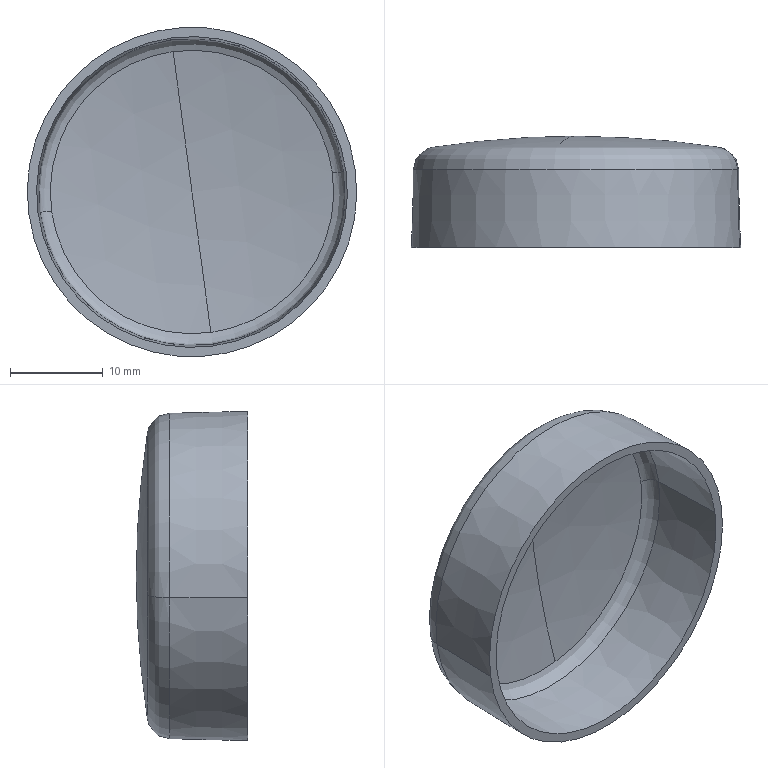Part | SolidWorks | features BaseBody 1 | 1 solid | 13 faces | box 35.5 x 12 x 35.5 mm | volume 1936 mm3 | cone 4 | torus 4 | sphere 4 | plane 1
STEP:
#1=CARTESIAN_POINT('',(53.884,-51.605,2.336));
#2=VERTEX_POINT('',#1);
#3=CARTESIAN_POINT('',(19.116,-51.605,-2.336));
#4=VERTEX_POINT('',#3);
#5=CARTESIAN_POINT('',(36.5,-51.605,0.));
#6=DIRECTION('',(0.,1.,0.));
#7=DIRECTION('',(0.9911,0.,0.1332));
#8=AXIS2_PLACEMENT_3D('',#5,#6,#7);
#9=CIRCLE('',#8,17.54);
#10=EDGE_CURVE('',#2,#4,#9,.T.);
#11=ORIENTED_EDGE('',*,*,#10,.F.);
#12=CARTESIAN_POINT('',(54.092,-60.,2.364));
#13=VERTEX_POINT('',#12);
#14=CARTESIAN_POINT('',(54.092,-60.,2.364));
#15=DIRECTION('',(0.02477,-0.9997,0.003329));
#16=VECTOR('',#15,1000.);
#17=LINE('',#14,#16);
#18=EDGE_CURVE('',#2,#13,#17,.T.);
#19=ORIENTED_EDGE('',*,*,#18,.T.);
#20=CARTESIAN_POINT('',(18.908,-60.,-2.364));
#21=VERTEX_POINT('',#20);
#22=CARTESIAN_POINT('',(36.5,-60.,0.));
#23=DIRECTION('',(0.,1.,0.));
#24=DIRECTION('',(0.9911,0.,0.1332));
#25=AXIS2_PLACEMENT_3D('',#22,#23,#24);
#26=CIRCLE('',#25,17.75);
#27=EDGE_CURVE('',#13,#21,#26,.T.);
#28=ORIENTED_EDGE('',*,*,#27,.T.);
#29=CARTESIAN_POINT('',(18.908,-60.,-2.364));
#30=DIRECTION('',(-0.02477,-0.9997,-0.003329));
#31=VECTOR('',#30,1000.);
#32=LINE('',#29,#31);
#33=EDGE_CURVE('',#4,#21,#32,.T.);
#34=ORIENTED_EDGE('',*,*,#33,.F.);
#35=EDGE_LOOP('',(#11,#19,#28,#34));
#36=FACE_OUTER_BOUND('',#35,.T.);
#37=CARTESIAN_POINT('',(36.5,-60.,0.));
#38=DIRECTION('',(0.,-1.,0.));
#39=DIRECTION('',(-0.9911,0.,-0.1332));
#40=AXIS2_PLACEMENT_3D('',#37,#38,#39);
#41=CONICAL_SURFACE('',#40,17.75,0.02499);
#42=ADVANCED_FACE('',(#36),#41,.T.);
#43=CARTESIAN_POINT('',(20.107,-51.63,-2.203));
#44=VERTEX_POINT('',#43);
#45=CARTESIAN_POINT('',(52.893,-51.63,2.203));
#46=VERTEX_POINT('',#45);
#47=CARTESIAN_POINT('',(36.5,-51.63,0.));
#48=DIRECTION('',(0.,1.,0.));
#49=DIRECTION('',(0.9911,0.,0.1332));
#50=AXIS2_PLACEMENT_3D('',#47,#48,#49);
#51=CIRCLE('',#50,16.54);
#52=EDGE_CURVE('',#44,#46,#51,.T.);
#53=ORIENTED_EDGE('',*,*,#52,.T.);
#54=CARTESIAN_POINT('',(53.1,-60.,2.231));
#55=VERTEX_POINT('',#54);
#56=CARTESIAN_POINT('',(52.893,-51.63,2.203));
#57=DIRECTION('',(0.02477,-0.9997,0.003329));
#58=VECTOR('',#57,1000.);
#59=LINE('',#56,#58);
#60=EDGE_CURVE('',#46,#55,#59,.T.);
#61=ORIENTED_EDGE('',*,*,#60,.T.);
#62=CARTESIAN_POINT('',(19.9,-60.,-2.231));
#63=VERTEX_POINT('',#62);
#64=CARTESIAN_POINT('',(36.5,-60.,0.));
#65=DIRECTION('',(0.,1.,0.));
#66=DIRECTION('',(0.9911,0.,0.1332));
#67=AXIS2_PLACEMENT_3D('',#64,#65,#66);
#68=CIRCLE('',#67,16.75);
#69=EDGE_CURVE('',#63,#55,#68,.T.);
#70=ORIENTED_EDGE('',*,*,#69,.F.);
#71=CARTESIAN_POINT('',(20.107,-51.63,-2.203));
#72=DIRECTION('',(-0.02477,-0.9997,-0.003329));
#73=VECTOR('',#72,1000.);
#74=LINE('',#71,#73);
#75=EDGE_CURVE('',#44,#63,#74,.T.);
#76=ORIENTED_EDGE('',*,*,#75,.F.);
#77=EDGE_LOOP('',(#53,#61,#70,#76));
#78=FACE_OUTER_BOUND('',#77,.T.);
#79=CARTESIAN_POINT('',(36.5,-51.63,0.));
#80=DIRECTION('',(0.,-1.,0.));
#81=DIRECTION('',(-0.9911,0.,-0.1332));
#82=AXIS2_PLACEMENT_3D('',#79,#80,#81);
#83=CONICAL_SURFACE('',#82,16.54,0.02499);
#84=ADVANCED_FACE('',(#78),#83,.F.);
#85=ORIENTED_EDGE('',*,*,#52,.F.);
#86=CARTESIAN_POINT('',(21.364,-50.185,-2.034));
#87=VERTEX_POINT('',#86);
#88=CARTESIAN_POINT('',(21.593,-51.667,-2.003));
#89=DIRECTION('',(0.1332,0.,-0.9911));
#90=DIRECTION('',(-0.9911,0.,-0.1332));
#91=AXIS2_PLACEMENT_3D('',#88,#89,#90);
#92=CIRCLE('',#91,1.5);
#93=EDGE_CURVE('',#44,#87,#92,.T.);
#94=ORIENTED_EDGE('',*,*,#93,.T.);
#95=CARTESIAN_POINT('',(34.466,-50.185,15.136));
#96=VERTEX_POINT('',#95);
#97=CARTESIAN_POINT('',(36.5,-50.185,0.));
#98=DIRECTION('',(0.,1.,0.));
#99=DIRECTION('',(0.9911,0.,0.1332));
#100=AXIS2_PLACEMENT_3D('',#97,#98,#99);
#101=CIRCLE('',#100,15.272);
#102=EDGE_CURVE('',#87,#96,#101,.T.);
#103=ORIENTED_EDGE('',*,*,#102,.T.);
#104=CARTESIAN_POINT('',(51.636,-50.185,2.034));
#105=VERTEX_POINT('',#104);
#106=CARTESIAN_POINT('',(36.5,-50.185,0.));
#107=DIRECTION('',(0.,1.,0.));
#108=DIRECTION('',(0.9911,0.,0.1332));
#109=AXIS2_PLACEMENT_3D('',#106,#107,#108);
#110=CIRCLE('',#109,15.272);
#111=EDGE_CURVE('',#96,#105,#110,.T.);
#112=ORIENTED_EDGE('',*,*,#111,.T.);
#113=CARTESIAN_POINT('',(51.407,-51.667,2.003));
#114=DIRECTION('',(-0.1332,0.,0.9911));
#115=DIRECTION('',(0.9911,0.,0.1332));
#116=AXIS2_PLACEMENT_3D('',#113,#114,#115);
#117=CIRCLE('',#116,1.5);
#118=EDGE_CURVE('',#46,#105,#117,.T.);
#119=ORIENTED_EDGE('',*,*,#118,.F.);
#120=EDGE_LOOP('',(#85,#94,#103,#112,#119));
#121=FACE_OUTER_BOUND('',#120,.T.);
#122=CARTESIAN_POINT('',(36.5,-51.667,0.));
#123=DIRECTION('',(0.,1.,0.));
#124=DIRECTION('',(0.9911,0.,0.1332));
#125=AXIS2_PLACEMENT_3D('',#122,#123,#124);
#126=TOROIDAL_SURFACE('',#125,15.041,1.5);
#127=ADVANCED_FACE('',(#121),#126,.F.);
#128=CARTESIAN_POINT('',(38.534,-50.185,-15.136));
#129=VERTEX_POINT('',#128);
#130=CARTESIAN_POINT('',(36.5,-50.185,0.));
#131=DIRECTION('',(0.,1.,0.));
#132=DIRECTION('',(0.9911,0.,0.1332));
#133=AXIS2_PLACEMENT_3D('',#130,#131,#132);
#134=CIRCLE('',#133,15.272);
#135=EDGE_CURVE('',#129,#87,#134,.T.);
#136=ORIENTED_EDGE('',*,*,#135,.F.);
#137=CARTESIAN_POINT('',(36.5,-49.,0.));
#138=VERTEX_POINT('',#137);
#139=CARTESIAN_POINT('',(36.5,-148.,0.));
#140=DIRECTION('',(0.9911,0.,0.1332));
#141=DIRECTION('',(0.1332,0.,-0.9911));
#142=AXIS2_PLACEMENT_3D('',#139,#140,#141);
#143=CIRCLE('',#142,99.);
#144=EDGE_CURVE('',#129,#138,#143,.T.);
#145=ORIENTED_EDGE('',*,*,#144,.T.);
#146=CARTESIAN_POINT('',(36.5,-148.,0.));
#147=DIRECTION('',(-0.9911,0.,-0.1332));
#148=DIRECTION('',(-0.1332,0.,0.9911));
#149=AXIS2_PLACEMENT_3D('',#146,#147,#148);
#150=CIRCLE('',#149,99.);
#151=EDGE_CURVE('',#96,#138,#150,.T.);
#152=ORIENTED_EDGE('',*,*,#151,.F.);
#153=ORIENTED_EDGE('',*,*,#102,.F.);
#154=EDGE_LOOP('',(#136,#145,#152,#153));
#155=FACE_OUTER_BOUND('',#154,.T.);
#156=CARTESIAN_POINT('',(36.5,-148.,0.));
#157=DIRECTION('',(0.9911,0.,0.1332));
#158=DIRECTION('',(-0.1332,0.,0.9911));
#159=AXIS2_PLACEMENT_3D('',#156,#157,#158);
#160=SPHERICAL_SURFACE('',#159,99.);
#161=ADVANCED_FACE('',(#155),#160,.F.);
#162=CARTESIAN_POINT('',(21.211,-49.197,-2.055));
#163=VERTEX_POINT('',#162);
#164=CARTESIAN_POINT('',(34.445,-49.197,15.289));
#165=VERTEX_POINT('',#164);
#166=CARTESIAN_POINT('',(36.5,-49.197,0.));
#167=DIRECTION('',(0.,1.,0.));
#168=DIRECTION('',(0.9911,0.,0.1332));
#169=AXIS2_PLACEMENT_3D('',#166,#167,#168);
#170=CIRCLE('',#169,15.427);
#171=EDGE_CURVE('',#163,#165,#170,.T.);
#172=ORIENTED_EDGE('',*,*,#171,.T.);
#173=CARTESIAN_POINT('',(36.5,-48.,0.));
#174=VERTEX_POINT('',#173);
#175=CARTESIAN_POINT('',(36.5,-148.,0.));
#176=DIRECTION('',(-0.9911,0.,-0.1332));
#177=DIRECTION('',(-0.1332,0.,0.9911));
#178=AXIS2_PLACEMENT_3D('',#175,#176,#177);
#179=CIRCLE('',#178,100.);
#180=EDGE_CURVE('',#165,#174,#179,.T.);
#181=ORIENTED_EDGE('',*,*,#180,.T.);
#182=CARTESIAN_POINT('',(38.555,-49.197,-15.289));
#183=VERTEX_POINT('',#182);
#184=CARTESIAN_POINT('',(36.5,-148.,0.));
#185=DIRECTION('',(0.9911,0.,0.1332));
#186=DIRECTION('',(0.1332,0.,-0.9911));
#187=AXIS2_PLACEMENT_3D('',#184,#185,#186);
#188=CIRCLE('',#187,100.);
#189=EDGE_CURVE('',#183,#174,#188,.T.);
#190=ORIENTED_EDGE('',*,*,#189,.F.);
#191=CARTESIAN_POINT('',(36.5,-49.197,0.));
#192=DIRECTION('',(0.,1.,0.));
#193=DIRECTION('',(0.9911,0.,0.1332));
#194=AXIS2_PLACEMENT_3D('',#191,#192,#193);
#195=CIRCLE('',#194,15.427);
#196=EDGE_CURVE('',#183,#163,#195,.T.);
#197=ORIENTED_EDGE('',*,*,#196,.T.);
#198=EDGE_LOOP('',(#172,#181,#190,#197));
#199=FACE_OUTER_BOUND('',#198,.T.);
#200=CARTESIAN_POINT('',(36.5,-148.,0.));
#201=DIRECTION('',(-0.9911,0.,-0.1332));
#202=DIRECTION('',(0.1332,0.,-0.9911));
#203=AXIS2_PLACEMENT_3D('',#200,#201,#202);
#204=SPHERICAL_SURFACE('',#203,100.);
#205=ADVANCED_FACE('',(#199),#204,.T.);
#206=ORIENTED_EDGE('',*,*,#10,.T.);
#207=CARTESIAN_POINT('',(21.593,-51.667,-2.003));
#208=DIRECTION('',(0.1332,0.,-0.9911));
#209=DIRECTION('',(-0.9911,0.,-0.1332));
#210=AXIS2_PLACEMENT_3D('',#207,#208,#209);
#211=CIRCLE('',#210,2.5);
#212=EDGE_CURVE('',#4,#163,#211,.T.);
#213=ORIENTED_EDGE('',*,*,#212,.T.);
#214=ORIENTED_EDGE('',*,*,#196,.F.);
#215=CARTESIAN_POINT('',(51.789,-49.197,2.055));
#216=VERTEX_POINT('',#215);
#217=CARTESIAN_POINT('',(36.5,-49.197,0.));
#218=DIRECTION('',(0.,1.,0.));
#219=DIRECTION('',(0.9911,0.,0.1332));
#220=AXIS2_PLACEMENT_3D('',#217,#218,#219);
#221=CIRCLE('',#220,15.427);
#222=EDGE_CURVE('',#216,#183,#221,.T.);
#223=ORIENTED_EDGE('',*,*,#222,.F.);
#224=CARTESIAN_POINT('',(51.407,-51.667,2.003));
#225=DIRECTION('',(-0.1332,0.,0.9911));
#226=DIRECTION('',(0.9911,0.,0.1332));
#227=AXIS2_PLACEMENT_3D('',#224,#225,#226);
#228=CIRCLE('',#227,2.5);
#229=EDGE_CURVE('',#2,#216,#228,.T.);
#230=ORIENTED_EDGE('',*,*,#229,.F.);
#231=EDGE_LOOP('',(#206,#213,#214,#223,#230));
#232=FACE_OUTER_BOUND('',#231,.T.);
#233=CARTESIAN_POINT('',(36.5,-51.667,0.));
#234=DIRECTION('',(0.,1.,0.));
#235=DIRECTION('',(0.9911,0.,0.1332));
#236=AXIS2_PLACEMENT_3D('',#233,#234,#235);
#237=TOROIDAL_SURFACE('',#236,15.041,2.5);
#238=ADVANCED_FACE('',(#232),#237,.T.);
#239=ORIENTED_EDGE('',*,*,#212,.F.);
#240=CARTESIAN_POINT('',(36.5,-51.605,0.));
#241=DIRECTION('',(0.,1.,0.));
#242=DIRECTION('',(0.9911,0.,0.1332));
#243=AXIS2_PLACEMENT_3D('',#240,#241,#242);
#244=CIRCLE('',#243,17.54);
#245=EDGE_CURVE('',#4,#2,#244,.T.);
#246=ORIENTED_EDGE('',*,*,#245,.T.);
#247=ORIENTED_EDGE('',*,*,#229,.T.);
#248=CARTESIAN_POINT('',(36.5,-49.197,0.));
#249=DIRECTION('',(0.,1.,0.));
#250=DIRECTION('',(0.9911,0.,0.1332));
#251=AXIS2_PLACEMENT_3D('',#248,#249,#250);
#252=CIRCLE('',#251,15.427);
#253=EDGE_CURVE('',#165,#216,#252,.T.);
#254=ORIENTED_EDGE('',*,*,#253,.F.);
#255=ORIENTED_EDGE('',*,*,#171,.F.);
#256=EDGE_LOOP('',(#239,#246,#247,#254,#255));
#257=FACE_OUTER_BOUND('',#256,.T.);
#258=CARTESIAN_POINT('',(36.5,-51.667,0.));
#259=DIRECTION('',(0.,1.,0.));
#260=DIRECTION('',(0.9911,0.,0.1332));
#261=AXIS2_PLACEMENT_3D('',#258,#259,#260);
#262=TOROIDAL_SURFACE('',#261,15.041,2.5);
#263=ADVANCED_FACE('',(#257),#262,.T.);
#264=ORIENTED_EDGE('',*,*,#180,.F.);
#265=ORIENTED_EDGE('',*,*,#253,.T.);
#266=ORIENTED_EDGE('',*,*,#222,.T.);
#267=ORIENTED_EDGE('',*,*,#189,.T.);
#268=EDGE_LOOP('',(#264,#265,#266,#267));
#269=FACE_OUTER_BOUND('',#268,.T.);
#270=CARTESIAN_POINT('',(36.5,-148.,0.));
#271=DIRECTION('',(-0.9911,0.,-0.1332));
#272=DIRECTION('',(0.1332,0.,-0.9911));
#273=AXIS2_PLACEMENT_3D('',#270,#271,#272);
#274=SPHERICAL_SURFACE('',#273,100.);
#275=ADVANCED_FACE('',(#269),#274,.T.);
#276=ORIENTED_EDGE('',*,*,#144,.F.);
#277=CARTESIAN_POINT('',(36.5,-50.185,0.));
#278=DIRECTION('',(0.,1.,0.));
#279=DIRECTION('',(0.9911,0.,0.1332));
#280=AXIS2_PLACEMENT_3D('',#277,#278,#279);
#281=CIRCLE('',#280,15.272);
#282=EDGE_CURVE('',#105,#129,#281,.T.);
#283=ORIENTED_EDGE('',*,*,#282,.F.);
#284=ORIENTED_EDGE('',*,*,#111,.F.);
#285=ORIENTED_EDGE('',*,*,#151,.T.);
#286=EDGE_LOOP('',(#276,#283,#284,#285));
#287=FACE_OUTER_BOUND('',#286,.T.);
#288=CARTESIAN_POINT('',(36.5,-148.,0.));
#289=DIRECTION('',(0.9911,0.,0.1332));
#290=DIRECTION('',(-0.1332,0.,0.9911));
#291=AXIS2_PLACEMENT_3D('',#288,#289,#290);
#292=SPHERICAL_SURFACE('',#291,99.);
#293=ADVANCED_FACE('',(#287),#292,.F.);
#294=ORIENTED_EDGE('',*,*,#93,.F.);
#295=CARTESIAN_POINT('',(36.5,-51.63,0.));
#296=DIRECTION('',(0.,1.,0.));
#297=DIRECTION('',(0.9911,0.,0.1332));
#298=AXIS2_PLACEMENT_3D('',#295,#296,#297);
#299=CIRCLE('',#298,16.54);
#300=EDGE_CURVE('',#46,#44,#299,.T.);
#301=ORIENTED_EDGE('',*,*,#300,.F.);
#302=ORIENTED_EDGE('',*,*,#118,.T.);
#303=ORIENTED_EDGE('',*,*,#282,.T.);
#304=ORIENTED_EDGE('',*,*,#135,.T.);
#305=EDGE_LOOP('',(#294,#301,#302,#303,#304));
#306=FACE_OUTER_BOUND('',#305,.T.);
#307=CARTESIAN_POINT('',(36.5,-51.667,0.));
#308=DIRECTION('',(0.,1.,0.));
#309=DIRECTION('',(0.9911,0.,0.1332));
#310=AXIS2_PLACEMENT_3D('',#307,#308,#309);
#311=TOROIDAL_SURFACE('',#310,15.041,1.5);
#312=ADVANCED_FACE('',(#306),#311,.F.);
#313=ORIENTED_EDGE('',*,*,#60,.F.);
#314=ORIENTED_EDGE('',*,*,#300,.T.);
#315=ORIENTED_EDGE('',*,*,#75,.T.);
#316=CARTESIAN_POINT('',(36.5,-60.,0.));
#317=DIRECTION('',(0.,1.,0.));
#318=DIRECTION('',(0.9911,0.,0.1332));
#319=AXIS2_PLACEMENT_3D('',#316,#317,#318);
#320=CIRCLE('',#319,16.75);
#321=EDGE_CURVE('',#55,#63,#320,.T.);
#322=ORIENTED_EDGE('',*,*,#321,.F.);
#323=EDGE_LOOP('',(#313,#314,#315,#322));
#324=FACE_OUTER_BOUND('',#323,.T.);
#325=CARTESIAN_POINT('',(36.5,-51.63,0.));
#326=DIRECTION('',(0.,-1.,0.));
#327=DIRECTION('',(-0.9911,0.,-0.1332));
#328=AXIS2_PLACEMENT_3D('',#325,#326,#327);
#329=CONICAL_SURFACE('',#328,16.54,0.02499);
#330=ADVANCED_FACE('',(#324),#329,.F.);
#331=CARTESIAN_POINT('',(36.5,-60.,0.));
#332=DIRECTION('',(0.,1.,0.));
#333=DIRECTION('',(0.9911,0.,0.1332));
#334=AXIS2_PLACEMENT_3D('',#331,#332,#333);
#335=CIRCLE('',#334,17.75);
#336=EDGE_CURVE('',#21,#13,#335,.T.);
#337=ORIENTED_EDGE('',*,*,#336,.F.);
#338=ORIENTED_EDGE('',*,*,#27,.F.);
#339=EDGE_LOOP('',(#337,#338));
#340=FACE_OUTER_BOUND('',#339,.T.);
#341=ORIENTED_EDGE('',*,*,#69,.T.);
#342=ORIENTED_EDGE('',*,*,#321,.T.);
#343=EDGE_LOOP('',(#341,#342));
#344=FACE_BOUND('',#343,.T.);
#345=CARTESIAN_POINT('',(38.864,-60.,-17.592));
#346=DIRECTION('',(0.,1.,0.));
#347=DIRECTION('',(0.9911,0.,0.1332));
#348=AXIS2_PLACEMENT_3D('',#345,#346,#347);
#349=PLANE('',#348);
#350=ADVANCED_FACE('',(#340,#344),#349,.F.);
#351=ORIENTED_EDGE('',*,*,#18,.F.);
#352=ORIENTED_EDGE('',*,*,#245,.F.);
#353=ORIENTED_EDGE('',*,*,#33,.T.);
#354=ORIENTED_EDGE('',*,*,#336,.T.);
#355=EDGE_LOOP('',(#351,#352,#353,#354));
#356=FACE_OUTER_BOUND('',#355,.T.);
#357=CARTESIAN_POINT('',(36.5,-60.,0.));
#358=DIRECTION('',(0.,-1.,0.));
#359=DIRECTION('',(-0.9911,0.,-0.1332));
#360=AXIS2_PLACEMENT_3D('',#357,#358,#359);
#361=CONICAL_SURFACE('',#360,17.75,0.02499);
#362=ADVANCED_FACE('',(#356),#361,.T.);
#363=CLOSED_SHELL('',(#42,#84,#127,#161,#205,#238,#263,#275,#293,#312,#330,#350,#362));
#364=MANIFOLD_SOLID_BREP('',#363);
#365=CARTESIAN_POINT('',(0.,0.,0.));
#366=DIRECTION('',(0.,0.,1.));
#367=DIRECTION('',(1.,0.,0.));
#368=AXIS2_PLACEMENT_3D('',#365,#366,#367);
#369=(LENGTH_UNIT()NAMED_UNIT(*)SI_UNIT(.MILLI.,.METRE.));
#370=UNCERTAINTY_MEASURE_WITH_UNIT(LENGTH_MEASURE(0.00001),#369,'','');
#371=(NAMED_UNIT(*)PLANE_ANGLE_UNIT()SI_UNIT($,.RADIAN.));
#372=(NAMED_UNIT(*)SI_UNIT($,.STERADIAN.)SOLID_ANGLE_UNIT());
#373=(GEOMETRIC_REPRESENTATION_CONTEXT(3)GLOBAL_UNCERTAINTY_ASSIGNED_CONTEXT((#370))GLOBAL_UNIT_ASSIGNED_CONTEXT((#369,#371,#372))REPRESENTATION_CONTEXT('',''));
#374=ADVANCED_BREP_SHAPE_REPRESENTATION('',(#364,#368),#373);